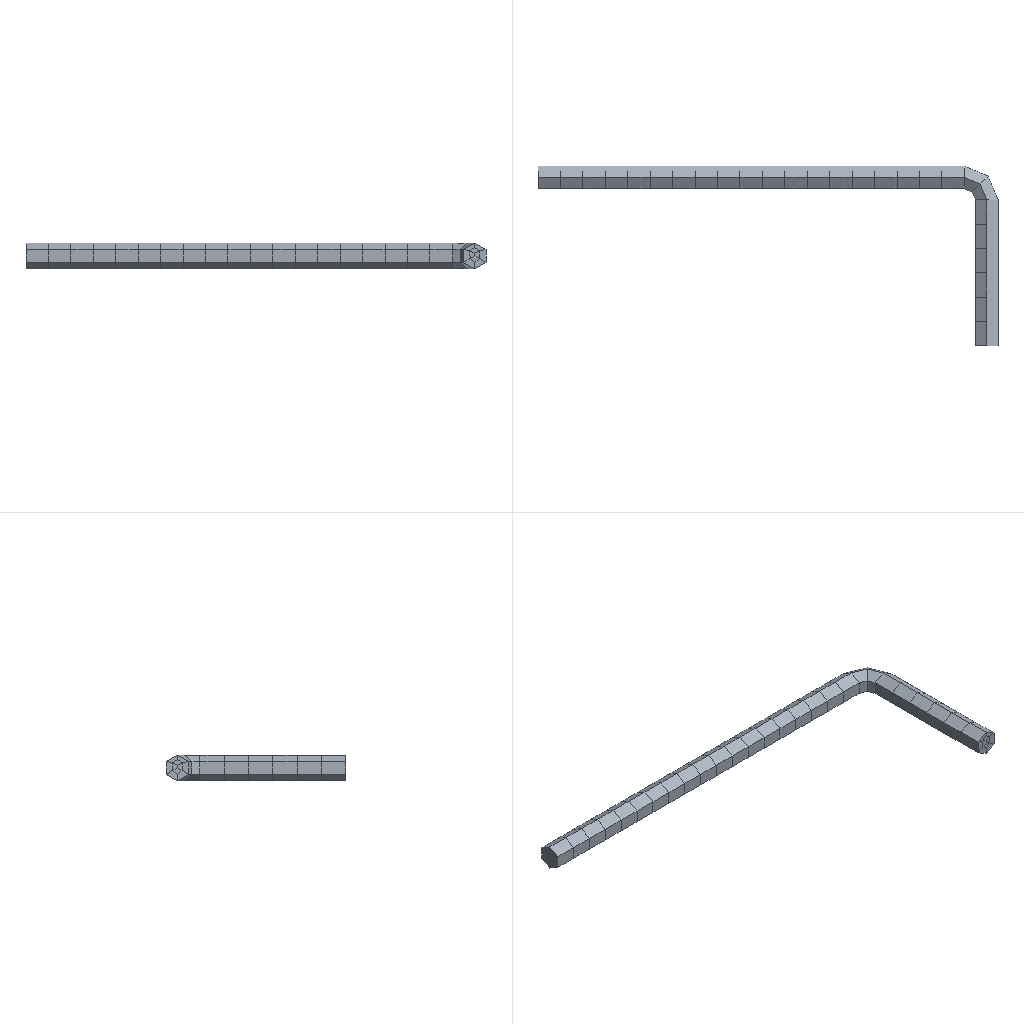Simulation study | ansys workbench
Set-up summary:
category,name,step,type,value,unit,region
solver,ansys_workbench
units,mm-N-s-tonne (MPa),,stated,"/units,MPA"
analysis,deck-1/LS1,,static
load_step,deck-1/LS1,deck-1/LS1,static,nsubst=1; time=1
analysis,deck-2/LS1,,static
load_step,deck-2/LS1,deck-2/LS1,static,nsubst=1; time=1
analysis,deck-3/LS1,,modal,method=lanb; n_modes=10
load_step,deck-3/LS1,deck-3/LS1,modal
mesh,deck-1.dat,,nodes,1414
mesh,deck-1.dat,,elements,327
element_type,SOLID186,,,270,,deck-1.dat
element_type,SURF154,,,57,,deck-1.dat
mesh,deck-2.dat,,nodes,1087
mesh,deck-2.dat,,elements,922
element_type,BEAM188,,,542,,deck-2.dat
element_type,SURF156,,,380,,deck-2.dat
mesh,deck-3.dat,,nodes,1414
mesh,deck-3.dat,,elements,270
element_type,SOLID186,,,270,,deck-3.dat
material,Structural Steel,,E,200000,tonne s^-2 mm^-1
material,Structural Steel,,nu,0.3
material,Structural Steel,,density,7.85e-09,tonne mm^-3
material,Structural Steel,,conductivity,60.5,tonne mm s^-3 C^-1
material,Structural Steel,,specific_heat,4.34e+08,mm^2 s^-2 C^-1
material,Structural Steel,,cte,1.2e-05,C^-1
material,Structural Steel,,permeability,10000
material,Structural Steel,,resistivity,0.00017,ohm mm
material,Structural Steel,,E,200000,tonne s^-2 mm^-1
material,Structural Steel,,nu,0.3
material,Structural Steel,,density,7.85e-09,tonne mm^-3
material,Structural Steel,,conductivity,60.5,tonne mm s^-3 C^-1
material,Structural Steel,,specific_heat,4.34e+08,mm^2 s^-2 C^-1
material,Structural Steel,,cte,1.2e-05,C^-1
material,Structural Steel,,permeability,10000
material,Structural Steel,,resistivity,0.00017,ohm mm
material,Structural Steel,,E,200000,tonne s^-2 mm^-1
material,Structural Steel,,nu,0.3
material,Structural Steel,,density,7.85e-09,tonne mm^-3
material,Structural Steel,,conductivity,60.5,tonne mm s^-3 C^-1
material,Structural Steel,,specific_heat,4.34e+08,mm^2 s^-2 C^-1
material,Structural Steel,,cte,1.2e-05,C^-1
material,Structural Steel,,permeability,10000
material,Structural Steel,,resistivity,0.00017,ohm mm
load,Define Force Using Surface Effect Elements,deck-1/LS1,surface-effect pres face 3,-0.04558,,SURF154 #2
load,Define Force Using Surface Effect Elements,deck-1/LS1,surface-effect pres face 2,-0.01823,,SURF154 #3
load,Define Force Using Surface Effect Elements,deck-1/LS1,surface-effect pres face 3,-6.02588e-17,,SURF154 #3
load,Define Force Using Surface Effect Elements,deck-2/LS1,surface-effect pres face 3,-1.053,,SURF156 #4
bc,Fixed Supports,deck-1/model,fixed,[dofs=ALL],,_FIXEDSU
bc,Fixed Supports,deck-2/model,fixed,[dofs=ALL],,_FIXEDSU
named_set,_FIXEDSU,,node,37
named_set,_FIXEDSU,,node,1
Results summary:
result,analyses[0].index,,,1
result,analyses[0].system,,,SYS
result,analyses[0].deck,,,deck-1.dat
result,analyses[0].solve_status,,,completed
result,analyses[0].analysis_type,,,static
result,analyses[0].physics,,,mechanical
result,analyses[0].unit_system,,,"NMM: mm, ton, N, s, mV, mA, degC"
result,analyses[0].n_sets,,,1
result,analyses[0].load_steps[0].set,set=1,,1
result,analyses[0].load_steps[0].time_or_freq,set=1,,1
result,analyses[0].load_steps[0].max_displacement_magnitude,set=1,,2.64
result,analyses[0].load_steps[0].max_von_mises_nodal,set=1,,133.339
result,analyses[0].load_steps[0].reaction_force_sum_xyz[1],set=1,,2.51682e-06
result,analyses[0].load_steps[0].reaction_force_sum_xyz[2],set=1,,20
result,analyses[0].load_steps[0].reaction_force_sum_xyz[3],set=1,,100
result,analyses[1].index,,,2
result,analyses[1].system,,,SYS-1
result,analyses[1].deck,,,deck-2.dat
result,analyses[1].solve_status,,,terminated_with_error
result,analyses[1].note,,,no rst/rth in package
result,analyses[2].index,,,3
result,analyses[2].system,,,SYS-2
result,analyses[2].deck,,,deck-3.dat
result,analyses[2].solve_status,,,completed
result,analyses[2].analysis_type,,,modal
result,analyses[2].physics,,,mechanical
result,analyses[2].unit_system,,,"NMM: mm, ton, N, s, mV, mA, degC"
result,analyses[2].n_sets,,,10
result,analyses[2].modal_frequencies_hz[1],,,0
result,analyses[2].modal_frequencies_hz[2],,,0
result,analyses[2].modal_frequencies_hz[3],,,0
result,analyses[2].modal_frequencies_hz[4],,,0.00108
result,analyses[2].modal_frequencies_hz[5],,,0.003082
result,analyses[2].modal_frequencies_hz[6],,,0.01034
result,analyses[2].modal_frequencies_hz[7],,,651.825
result,analyses[2].modal_frequencies_hz[8],,,1046.62
result,analyses[2].modal_frequencies_hz[9],,,1412.35
result,analyses[2].modal_frequencies_hz[10],,,2860.11
result,geometry_export[0][0],,,.step
result,geometry_export[0][1],,,ok
result,geometry_export[0][2],,,1